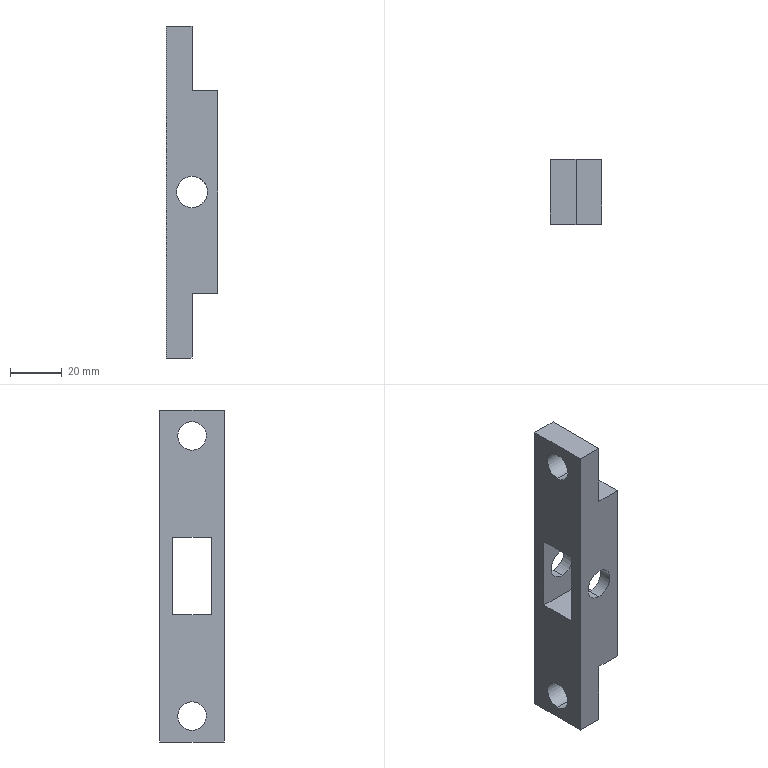Part | STEP file | Positioning_id1362_x_t | 1 solid | 22 faces | box 20 x 25 x 128 mm | volume 39468 mm3 | plane 14 | cylinder 8 | commonest cylinder face diameters 11 x4 12 x4